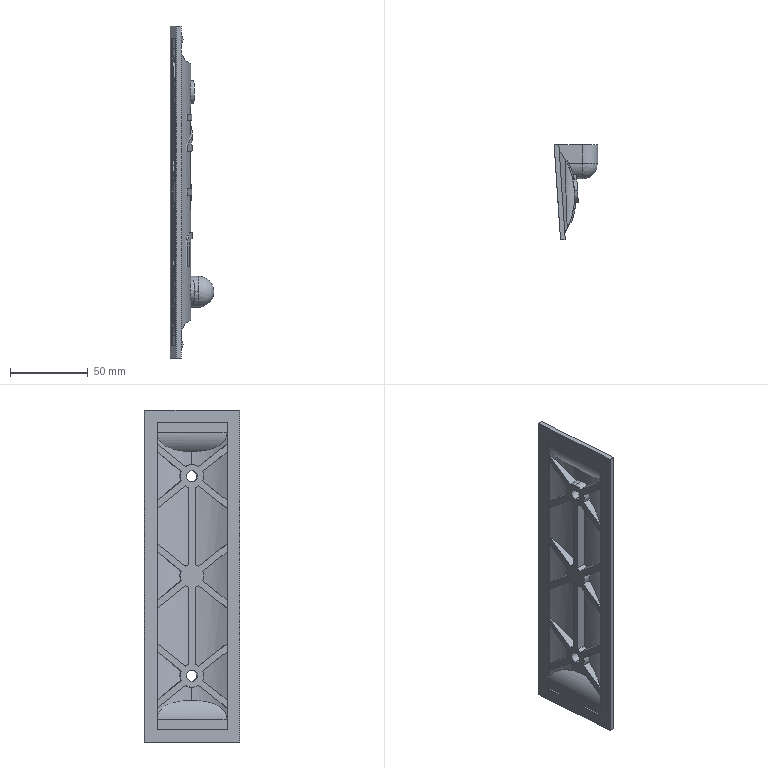Part | SolidWorks | features BaseBody 1 | 1 solid | 159 faces | box 27.993 x 61.065 x 213 mm | volume 66009 mm3 | plane 85 | cylinder 69 | cone 4 | sphere 1 | commonest cylinder face diameters 15 x20 88.135 x14 97.781 x8 20 x5 7 x4 10.5 x4